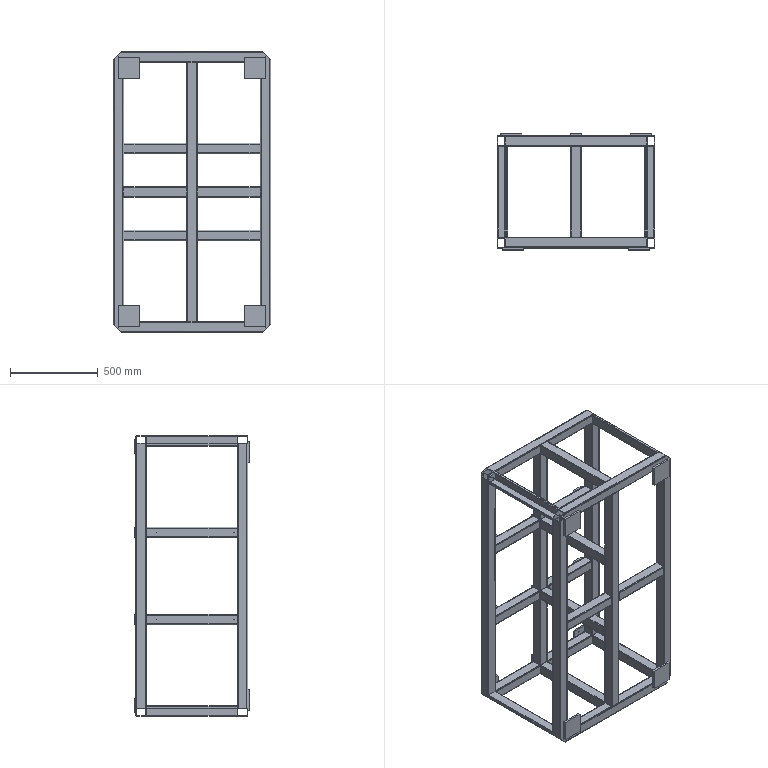Part | STEP file | Square tube frame_default<as machined> | 40 solids | 608 faces | box 896 x 660 x 1596 mm | volume 13190775 mm3 | plane 376 | cylinder 232 | commonest cylinder face diameters 4 x92 10 x92 6.8 x40 5 x8